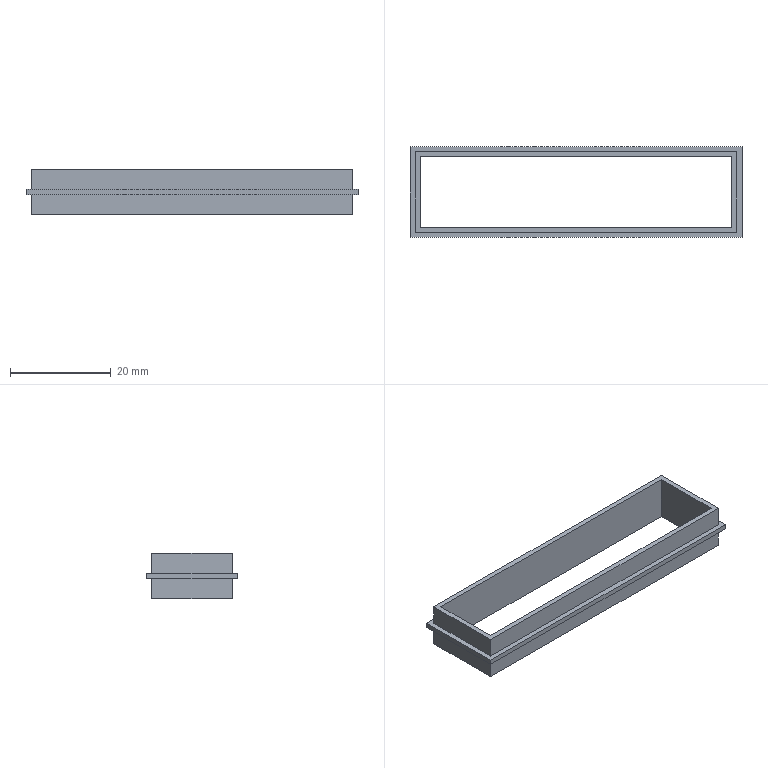Part | STEP file | 1-43.10 | 1 solid | 20 faces | box 66 x 18 x 9 mm | volume 1568 mm3 | plane 20
STEP:
#1=CARTESIAN_POINT('',(0.,0.,0.));
#2=DIRECTION('',(0.,0.,1.));
#3=DIRECTION('',(1.,0.,0.));
#4=AXIS2_PLACEMENT_3D('',#1,#2,#3);
#5=CARTESIAN_POINT('',(-32.,-8.,4.5));
#6=VERTEX_POINT('',#5);
#7=CARTESIAN_POINT('',(32.,-8.,4.5));
#8=VERTEX_POINT('',#7);
#9=CARTESIAN_POINT('',(-32.,-8.,4.5));
#10=DIRECTION('',(1.,0.,0.));
#11=VECTOR('',#10,1.);
#12=LINE('',#9,#11);
#13=CARTESIAN_POINT('',(0.,24.,4.5));
#14=DIRECTION('',(0.,0.,1.));
#15=DIRECTION('',(0.,1.,0.));
#16=AXIS2_PLACEMENT_3D('',#13,#14,#15);
#17=PLANE('',#16);
#18=CARTESIAN_POINT('',(-32.,32.));
#19=DIRECTION('',(0.,-1.));
#20=VECTOR('',#19,1.);
#21=LINE('',#18,#20);
#22=(GEOMETRIC_REPRESENTATION_CONTEXT(2)PARAMETRIC_REPRESENTATION_CONTEXT()REPRESENTATION_CONTEXT('',''));
#23=DEFINITIONAL_REPRESENTATION('',(#21),#22);
#24=PCURVE('',#17,#23);
#25=CARTESIAN_POINT('',(0.,-8.,0.));
#26=DIRECTION('',(0.,1.,0.));
#27=DIRECTION('',(1.,0.,0.));
#28=AXIS2_PLACEMENT_3D('',#25,#26,#27);
#29=PLANE('',#28);
#30=CARTESIAN_POINT('',(-32.,-4.5));
#31=DIRECTION('',(1.,0.));
#32=VECTOR('',#31,1.);
#33=LINE('',#30,#32);
#34=(GEOMETRIC_REPRESENTATION_CONTEXT(2)PARAMETRIC_REPRESENTATION_CONTEXT()REPRESENTATION_CONTEXT('',''));
#35=DEFINITIONAL_REPRESENTATION('',(#33),#34);
#36=PCURVE('',#29,#35);
#37=SURFACE_CURVE('',#12,(#24,#36),.PCURVE_S1.);
#38=EDGE_CURVE('',#6,#8,#37,.T.);
#39=ORIENTED_EDGE('',*,*,#38,.T.);
#40=CARTESIAN_POINT('',(32.,8.,4.5));
#41=VERTEX_POINT('',#40);
#42=CARTESIAN_POINT('',(32.,-8.,4.5));
#43=DIRECTION('',(0.,1.,0.));
#44=VECTOR('',#43,1.);
#45=LINE('',#42,#44);
#46=CARTESIAN_POINT('',(-32.,-32.));
#47=DIRECTION('',(1.,0.));
#48=VECTOR('',#47,1.);
#49=LINE('',#46,#48);
#50=(GEOMETRIC_REPRESENTATION_CONTEXT(2)PARAMETRIC_REPRESENTATION_CONTEXT()REPRESENTATION_CONTEXT('',''));
#51=DEFINITIONAL_REPRESENTATION('',(#49),#50);
#52=PCURVE('',#17,#51);
#53=CARTESIAN_POINT('',(32.,0.,0.));
#54=DIRECTION('',(-1.,0.,0.));
#55=DIRECTION('',(0.,1.,0.));
#56=AXIS2_PLACEMENT_3D('',#53,#54,#55);
#57=PLANE('',#56);
#58=CARTESIAN_POINT('',(-8.,-4.5));
#59=DIRECTION('',(1.,0.));
#60=VECTOR('',#59,1.);
#61=LINE('',#58,#60);
#62=(GEOMETRIC_REPRESENTATION_CONTEXT(2)PARAMETRIC_REPRESENTATION_CONTEXT()REPRESENTATION_CONTEXT('',''));
#63=DEFINITIONAL_REPRESENTATION('',(#61),#62);
#64=PCURVE('',#57,#63);
#65=SURFACE_CURVE('',#45,(#52,#64),.PCURVE_S1.);
#66=EDGE_CURVE('',#8,#41,#65,.T.);
#67=ORIENTED_EDGE('',*,*,#66,.T.);
#68=CARTESIAN_POINT('',(-32.,8.,4.5));
#69=VERTEX_POINT('',#68);
#70=CARTESIAN_POINT('',(32.,8.,4.5));
#71=DIRECTION('',(-1.,0.,0.));
#72=VECTOR('',#71,1.);
#73=LINE('',#70,#72);
#74=CARTESIAN_POINT('',(-16.,-32.));
#75=DIRECTION('',(0.,1.));
#76=VECTOR('',#75,1.);
#77=LINE('',#74,#76);
#78=(GEOMETRIC_REPRESENTATION_CONTEXT(2)PARAMETRIC_REPRESENTATION_CONTEXT()REPRESENTATION_CONTEXT('',''));
#79=DEFINITIONAL_REPRESENTATION('',(#77),#78);
#80=PCURVE('',#17,#79);
#81=CARTESIAN_POINT('',(0.,8.,0.));
#82=DIRECTION('',(0.,-1.,0.));
#83=DIRECTION('',(-1.,0.,0.));
#84=AXIS2_PLACEMENT_3D('',#81,#82,#83);
#85=PLANE('',#84);
#86=CARTESIAN_POINT('',(-32.,-4.5));
#87=DIRECTION('',(1.,0.));
#88=VECTOR('',#87,1.);
#89=LINE('',#86,#88);
#90=(GEOMETRIC_REPRESENTATION_CONTEXT(2)PARAMETRIC_REPRESENTATION_CONTEXT()REPRESENTATION_CONTEXT('',''));
#91=DEFINITIONAL_REPRESENTATION('',(#89),#90);
#92=PCURVE('',#85,#91);
#93=SURFACE_CURVE('',#73,(#80,#92),.PCURVE_S1.);
#94=EDGE_CURVE('',#41,#69,#93,.T.);
#95=ORIENTED_EDGE('',*,*,#94,.T.);
#96=CARTESIAN_POINT('',(-32.,8.,4.5));
#97=DIRECTION('',(0.,-1.,0.));
#98=VECTOR('',#97,1.);
#99=LINE('',#96,#98);
#100=CARTESIAN_POINT('',(-16.,32.));
#101=DIRECTION('',(-1.,0.));
#102=VECTOR('',#101,1.);
#103=LINE('',#100,#102);
#104=(GEOMETRIC_REPRESENTATION_CONTEXT(2)PARAMETRIC_REPRESENTATION_CONTEXT()REPRESENTATION_CONTEXT('',''));
#105=DEFINITIONAL_REPRESENTATION('',(#103),#104);
#106=PCURVE('',#17,#105);
#107=CARTESIAN_POINT('',(-32.,0.,0.));
#108=DIRECTION('',(1.,0.,0.));
#109=DIRECTION('',(0.,-1.,0.));
#110=AXIS2_PLACEMENT_3D('',#107,#108,#109);
#111=PLANE('',#110);
#112=CARTESIAN_POINT('',(-8.,-4.5));
#113=DIRECTION('',(1.,0.));
#114=VECTOR('',#113,1.);
#115=LINE('',#112,#114);
#116=(GEOMETRIC_REPRESENTATION_CONTEXT(2)PARAMETRIC_REPRESENTATION_CONTEXT()REPRESENTATION_CONTEXT('',''));
#117=DEFINITIONAL_REPRESENTATION('',(#115),#116);
#118=PCURVE('',#111,#117);
#119=SURFACE_CURVE('',#99,(#106,#118),.PCURVE_S1.);
#120=EDGE_CURVE('',#69,#6,#119,.T.);
#121=ORIENTED_EDGE('',*,*,#120,.T.);
#122=EDGE_LOOP('',(#39,#67,#95,#121));
#123=FACE_BOUND('',#122,.T.);
#124=CARTESIAN_POINT('',(31.,-7.,4.5));
#125=VERTEX_POINT('',#124);
#126=CARTESIAN_POINT('',(-31.,-7.,4.5));
#127=VERTEX_POINT('',#126);
#128=CARTESIAN_POINT('',(31.,-7.,4.5));
#129=DIRECTION('',(-1.,0.,0.));
#130=VECTOR('',#129,1.);
#131=LINE('',#128,#130);
#132=CARTESIAN_POINT('',(-31.,-31.));
#133=DIRECTION('',(0.,1.));
#134=VECTOR('',#133,1.);
#135=LINE('',#132,#134);
#136=(GEOMETRIC_REPRESENTATION_CONTEXT(2)PARAMETRIC_REPRESENTATION_CONTEXT()REPRESENTATION_CONTEXT('',''));
#137=DEFINITIONAL_REPRESENTATION('',(#135),#136);
#138=PCURVE('',#17,#137);
#139=CARTESIAN_POINT('',(0.,-7.,0.));
#140=DIRECTION('',(0.,-1.,0.));
#141=DIRECTION('',(-1.,0.,0.));
#142=AXIS2_PLACEMENT_3D('',#139,#140,#141);
#143=PLANE('',#142);
#144=CARTESIAN_POINT('',(-31.,-4.5));
#145=DIRECTION('',(1.,0.));
#146=VECTOR('',#145,1.);
#147=LINE('',#144,#146);
#148=(GEOMETRIC_REPRESENTATION_CONTEXT(2)PARAMETRIC_REPRESENTATION_CONTEXT()REPRESENTATION_CONTEXT('',''));
#149=DEFINITIONAL_REPRESENTATION('',(#147),#148);
#150=PCURVE('',#143,#149);
#151=SURFACE_CURVE('',#131,(#138,#150),.PCURVE_S1.);
#152=EDGE_CURVE('',#125,#127,#151,.T.);
#153=ORIENTED_EDGE('',*,*,#152,.T.);
#154=CARTESIAN_POINT('',(-31.,7.,4.5));
#155=VERTEX_POINT('',#154);
#156=CARTESIAN_POINT('',(-31.,-7.,4.5));
#157=DIRECTION('',(0.,1.,0.));
#158=VECTOR('',#157,1.);
#159=LINE('',#156,#158);
#160=CARTESIAN_POINT('',(-31.,31.));
#161=DIRECTION('',(1.,0.));
#162=VECTOR('',#161,1.);
#163=LINE('',#160,#162);
#164=(GEOMETRIC_REPRESENTATION_CONTEXT(2)PARAMETRIC_REPRESENTATION_CONTEXT()REPRESENTATION_CONTEXT('',''));
#165=DEFINITIONAL_REPRESENTATION('',(#163),#164);
#166=PCURVE('',#17,#165);
#167=CARTESIAN_POINT('',(-31.,0.,0.));
#168=DIRECTION('',(-1.,0.,0.));
#169=DIRECTION('',(0.,1.,0.));
#170=AXIS2_PLACEMENT_3D('',#167,#168,#169);
#171=PLANE('',#170);
#172=CARTESIAN_POINT('',(-7.,-4.5));
#173=DIRECTION('',(1.,0.));
#174=VECTOR('',#173,1.);
#175=LINE('',#172,#174);
#176=(GEOMETRIC_REPRESENTATION_CONTEXT(2)PARAMETRIC_REPRESENTATION_CONTEXT()REPRESENTATION_CONTEXT('',''));
#177=DEFINITIONAL_REPRESENTATION('',(#175),#176);
#178=PCURVE('',#171,#177);
#179=SURFACE_CURVE('',#159,(#166,#178),.PCURVE_S1.);
#180=EDGE_CURVE('',#127,#155,#179,.T.);
#181=ORIENTED_EDGE('',*,*,#180,.T.);
#182=CARTESIAN_POINT('',(31.,7.,4.5));
#183=VERTEX_POINT('',#182);
#184=CARTESIAN_POINT('',(-31.,7.,4.5));
#185=DIRECTION('',(1.,0.,0.));
#186=VECTOR('',#185,1.);
#187=LINE('',#184,#186);
#188=CARTESIAN_POINT('',(-17.,31.));
#189=DIRECTION('',(0.,-1.));
#190=VECTOR('',#189,1.);
#191=LINE('',#188,#190);
#192=(GEOMETRIC_REPRESENTATION_CONTEXT(2)PARAMETRIC_REPRESENTATION_CONTEXT()REPRESENTATION_CONTEXT('',''));
#193=DEFINITIONAL_REPRESENTATION('',(#191),#192);
#194=PCURVE('',#17,#193);
#195=CARTESIAN_POINT('',(0.,7.,0.));
#196=DIRECTION('',(0.,1.,0.));
#197=DIRECTION('',(1.,0.,0.));
#198=AXIS2_PLACEMENT_3D('',#195,#196,#197);
#199=PLANE('',#198);
#200=CARTESIAN_POINT('',(-31.,-4.5));
#201=DIRECTION('',(1.,0.));
#202=VECTOR('',#201,1.);
#203=LINE('',#200,#202);
#204=(GEOMETRIC_REPRESENTATION_CONTEXT(2)PARAMETRIC_REPRESENTATION_CONTEXT()REPRESENTATION_CONTEXT('',''));
#205=DEFINITIONAL_REPRESENTATION('',(#203),#204);
#206=PCURVE('',#199,#205);
#207=SURFACE_CURVE('',#187,(#194,#206),.PCURVE_S1.);
#208=EDGE_CURVE('',#155,#183,#207,.T.);
#209=ORIENTED_EDGE('',*,*,#208,.T.);
#210=CARTESIAN_POINT('',(31.,7.,4.5));
#211=DIRECTION('',(0.,-1.,0.));
#212=VECTOR('',#211,1.);
#213=LINE('',#210,#212);
#214=CARTESIAN_POINT('',(-17.,-31.));
#215=DIRECTION('',(-1.,0.));
#216=VECTOR('',#215,1.);
#217=LINE('',#214,#216);
#218=(GEOMETRIC_REPRESENTATION_CONTEXT(2)PARAMETRIC_REPRESENTATION_CONTEXT()REPRESENTATION_CONTEXT('',''));
#219=DEFINITIONAL_REPRESENTATION('',(#217),#218);
#220=PCURVE('',#17,#219);
#221=CARTESIAN_POINT('',(31.,0.,0.));
#222=DIRECTION('',(1.,0.,0.));
#223=DIRECTION('',(0.,-1.,0.));
#224=AXIS2_PLACEMENT_3D('',#221,#222,#223);
#225=PLANE('',#224);
#226=CARTESIAN_POINT('',(-7.,-4.5));
#227=DIRECTION('',(1.,0.));
#228=VECTOR('',#227,1.);
#229=LINE('',#226,#228);
#230=(GEOMETRIC_REPRESENTATION_CONTEXT(2)PARAMETRIC_REPRESENTATION_CONTEXT()REPRESENTATION_CONTEXT('',''));
#231=DEFINITIONAL_REPRESENTATION('',(#229),#230);
#232=PCURVE('',#225,#231);
#233=SURFACE_CURVE('',#213,(#220,#232),.PCURVE_S1.);
#234=EDGE_CURVE('',#183,#125,#233,.T.);
#235=ORIENTED_EDGE('',*,*,#234,.T.);
#236=EDGE_LOOP('',(#153,#181,#209,#235));
#237=FACE_BOUND('',#236,.T.);
#238=ADVANCED_FACE('',(#123,#237),#17,.T.);
#239=CARTESIAN_POINT('',(-32.,-8.,-4.5));
#240=VERTEX_POINT('',#239);
#241=CARTESIAN_POINT('',(32.,-8.,-4.5));
#242=VERTEX_POINT('',#241);
#243=CARTESIAN_POINT('',(-32.,-8.,-4.5));
#244=DIRECTION('',(1.,0.,0.));
#245=VECTOR('',#244,1.);
#246=LINE('',#243,#245);
#247=CARTESIAN_POINT('',(0.,24.,-4.5));
#248=DIRECTION('',(0.,0.,1.));
#249=DIRECTION('',(0.,1.,0.));
#250=AXIS2_PLACEMENT_3D('',#247,#248,#249);
#251=PLANE('',#250);
#252=CARTESIAN_POINT('',(-32.,32.));
#253=DIRECTION('',(0.,-1.));
#254=VECTOR('',#253,1.);
#255=LINE('',#252,#254);
#256=(GEOMETRIC_REPRESENTATION_CONTEXT(2)PARAMETRIC_REPRESENTATION_CONTEXT()REPRESENTATION_CONTEXT('',''));
#257=DEFINITIONAL_REPRESENTATION('',(#255),#256);
#258=PCURVE('',#251,#257);
#259=CARTESIAN_POINT('',(0.,-8.,0.));
#260=DIRECTION('',(0.,1.,0.));
#261=DIRECTION('',(1.,0.,0.));
#262=AXIS2_PLACEMENT_3D('',#259,#260,#261);
#263=PLANE('',#262);
#264=CARTESIAN_POINT('',(-32.,4.5));
#265=DIRECTION('',(1.,0.));
#266=VECTOR('',#265,1.);
#267=LINE('',#264,#266);
#268=(GEOMETRIC_REPRESENTATION_CONTEXT(2)PARAMETRIC_REPRESENTATION_CONTEXT()REPRESENTATION_CONTEXT('',''));
#269=DEFINITIONAL_REPRESENTATION('',(#267),#268);
#270=PCURVE('',#263,#269);
#271=SURFACE_CURVE('',#246,(#258,#270),.PCURVE_S1.);
#272=EDGE_CURVE('',#240,#242,#271,.T.);
#273=ORIENTED_EDGE('',*,*,#272,.T.);
#274=CARTESIAN_POINT('',(32.,8.,-4.5));
#275=VERTEX_POINT('',#274);
#276=CARTESIAN_POINT('',(32.,-8.,-4.5));
#277=DIRECTION('',(0.,1.,0.));
#278=VECTOR('',#277,1.);
#279=LINE('',#276,#278);
#280=CARTESIAN_POINT('',(-32.,-32.));
#281=DIRECTION('',(1.,0.));
#282=VECTOR('',#281,1.);
#283=LINE('',#280,#282);
#284=(GEOMETRIC_REPRESENTATION_CONTEXT(2)PARAMETRIC_REPRESENTATION_CONTEXT()REPRESENTATION_CONTEXT('',''));
#285=DEFINITIONAL_REPRESENTATION('',(#283),#284);
#286=PCURVE('',#251,#285);
#287=CARTESIAN_POINT('',(32.,0.,0.));
#288=DIRECTION('',(-1.,0.,0.));
#289=DIRECTION('',(0.,1.,0.));
#290=AXIS2_PLACEMENT_3D('',#287,#288,#289);
#291=PLANE('',#290);
#292=CARTESIAN_POINT('',(-8.,4.5));
#293=DIRECTION('',(1.,0.));
#294=VECTOR('',#293,1.);
#295=LINE('',#292,#294);
#296=(GEOMETRIC_REPRESENTATION_CONTEXT(2)PARAMETRIC_REPRESENTATION_CONTEXT()REPRESENTATION_CONTEXT('',''));
#297=DEFINITIONAL_REPRESENTATION('',(#295),#296);
#298=PCURVE('',#291,#297);
#299=SURFACE_CURVE('',#279,(#286,#298),.PCURVE_S1.);
#300=EDGE_CURVE('',#242,#275,#299,.T.);
#301=ORIENTED_EDGE('',*,*,#300,.T.);
#302=CARTESIAN_POINT('',(-32.,8.,-4.5));
#303=VERTEX_POINT('',#302);
#304=CARTESIAN_POINT('',(32.,8.,-4.5));
#305=DIRECTION('',(-1.,0.,0.));
#306=VECTOR('',#305,1.);
#307=LINE('',#304,#306);
#308=CARTESIAN_POINT('',(-16.,-32.));
#309=DIRECTION('',(0.,1.));
#310=VECTOR('',#309,1.);
#311=LINE('',#308,#310);
#312=(GEOMETRIC_REPRESENTATION_CONTEXT(2)PARAMETRIC_REPRESENTATION_CONTEXT()REPRESENTATION_CONTEXT('',''));
#313=DEFINITIONAL_REPRESENTATION('',(#311),#312);
#314=PCURVE('',#251,#313);
#315=CARTESIAN_POINT('',(0.,8.,0.));
#316=DIRECTION('',(0.,-1.,0.));
#317=DIRECTION('',(-1.,0.,0.));
#318=AXIS2_PLACEMENT_3D('',#315,#316,#317);
#319=PLANE('',#318);
#320=CARTESIAN_POINT('',(-32.,4.5));
#321=DIRECTION('',(1.,0.));
#322=VECTOR('',#321,1.);
#323=LINE('',#320,#322);
#324=(GEOMETRIC_REPRESENTATION_CONTEXT(2)PARAMETRIC_REPRESENTATION_CONTEXT()REPRESENTATION_CONTEXT('',''));
#325=DEFINITIONAL_REPRESENTATION('',(#323),#324);
#326=PCURVE('',#319,#325);
#327=SURFACE_CURVE('',#307,(#314,#326),.PCURVE_S1.);
#328=EDGE_CURVE('',#275,#303,#327,.T.);
#329=ORIENTED_EDGE('',*,*,#328,.T.);
#330=CARTESIAN_POINT('',(-32.,8.,-4.5));
#331=DIRECTION('',(0.,-1.,0.));
#332=VECTOR('',#331,1.);
#333=LINE('',#330,#332);
#334=CARTESIAN_POINT('',(-16.,32.));
#335=DIRECTION('',(-1.,0.));
#336=VECTOR('',#335,1.);
#337=LINE('',#334,#336);
#338=(GEOMETRIC_REPRESENTATION_CONTEXT(2)PARAMETRIC_REPRESENTATION_CONTEXT()REPRESENTATION_CONTEXT('',''));
#339=DEFINITIONAL_REPRESENTATION('',(#337),#338);
#340=PCURVE('',#251,#339);
#341=CARTESIAN_POINT('',(-32.,0.,0.));
#342=DIRECTION('',(1.,0.,0.));
#343=DIRECTION('',(0.,-1.,0.));
#344=AXIS2_PLACEMENT_3D('',#341,#342,#343);
#345=PLANE('',#344);
#346=CARTESIAN_POINT('',(-8.,4.5));
#347=DIRECTION('',(1.,0.));
#348=VECTOR('',#347,1.);
#349=LINE('',#346,#348);
#350=(GEOMETRIC_REPRESENTATION_CONTEXT(2)PARAMETRIC_REPRESENTATION_CONTEXT()REPRESENTATION_CONTEXT('',''));
#351=DEFINITIONAL_REPRESENTATION('',(#349),#350);
#352=PCURVE('',#345,#351);
#353=SURFACE_CURVE('',#333,(#340,#352),.PCURVE_S1.);
#354=EDGE_CURVE('',#303,#240,#353,.T.);
#355=ORIENTED_EDGE('',*,*,#354,.T.);
#356=EDGE_LOOP('',(#273,#301,#329,#355));
#357=FACE_BOUND('',#356,.F.);
#358=CARTESIAN_POINT('',(31.,-7.,-4.5));
#359=VERTEX_POINT('',#358);
#360=CARTESIAN_POINT('',(-31.,-7.,-4.5));
#361=VERTEX_POINT('',#360);
#362=CARTESIAN_POINT('',(31.,-7.,-4.5));
#363=DIRECTION('',(-1.,0.,0.));
#364=VECTOR('',#363,1.);
#365=LINE('',#362,#364);
#366=CARTESIAN_POINT('',(-31.,-31.));
#367=DIRECTION('',(0.,1.));
#368=VECTOR('',#367,1.);
#369=LINE('',#366,#368);
#370=(GEOMETRIC_REPRESENTATION_CONTEXT(2)PARAMETRIC_REPRESENTATION_CONTEXT()REPRESENTATION_CONTEXT('',''));
#371=DEFINITIONAL_REPRESENTATION('',(#369),#370);
#372=PCURVE('',#251,#371);
#373=CARTESIAN_POINT('',(-31.,4.5));
#374=DIRECTION('',(1.,0.));
#375=VECTOR('',#374,1.);
#376=LINE('',#373,#375);
#377=(GEOMETRIC_REPRESENTATION_CONTEXT(2)PARAMETRIC_REPRESENTATION_CONTEXT()REPRESENTATION_CONTEXT('',''));
#378=DEFINITIONAL_REPRESENTATION('',(#376),#377);
#379=PCURVE('',#143,#378);
#380=SURFACE_CURVE('',#365,(#372,#379),.PCURVE_S1.);
#381=EDGE_CURVE('',#359,#361,#380,.T.);
#382=ORIENTED_EDGE('',*,*,#381,.T.);
#383=CARTESIAN_POINT('',(-31.,7.,-4.5));
#384=VERTEX_POINT('',#383);
#385=CARTESIAN_POINT('',(-31.,-7.,-4.5));
#386=DIRECTION('',(0.,1.,0.));
#387=VECTOR('',#386,1.);
#388=LINE('',#385,#387);
#389=CARTESIAN_POINT('',(-31.,31.));
#390=DIRECTION('',(1.,0.));
#391=VECTOR('',#390,1.);
#392=LINE('',#389,#391);
#393=(GEOMETRIC_REPRESENTATION_CONTEXT(2)PARAMETRIC_REPRESENTATION_CONTEXT()REPRESENTATION_CONTEXT('',''));
#394=DEFINITIONAL_REPRESENTATION('',(#392),#393);
#395=PCURVE('',#251,#394);
#396=CARTESIAN_POINT('',(-7.,4.5));
#397=DIRECTION('',(1.,0.));
#398=VECTOR('',#397,1.);
#399=LINE('',#396,#398);
#400=(GEOMETRIC_REPRESENTATION_CONTEXT(2)PARAMETRIC_REPRESENTATION_CONTEXT()REPRESENTATION_CONTEXT('',''));
#401=DEFINITIONAL_REPRESENTATION('',(#399),#400);
#402=PCURVE('',#171,#401);
#403=SURFACE_CURVE('',#388,(#395,#402),.PCURVE_S1.);
#404=EDGE_CURVE('',#361,#384,#403,.T.);
#405=ORIENTED_EDGE('',*,*,#404,.T.);
#406=CARTESIAN_POINT('',(31.,7.,-4.5));
#407=VERTEX_POINT('',#406);
#408=CARTESIAN_POINT('',(-31.,7.,-4.5));
#409=DIRECTION('',(1.,0.,0.));
#410=VECTOR('',#409,1.);
#411=LINE('',#408,#410);
#412=CARTESIAN_POINT('',(-17.,31.));
#413=DIRECTION('',(0.,-1.));
#414=VECTOR('',#413,1.);
#415=LINE('',#412,#414);
#416=(GEOMETRIC_REPRESENTATION_CONTEXT(2)PARAMETRIC_REPRESENTATION_CONTEXT()REPRESENTATION_CONTEXT('',''));
#417=DEFINITIONAL_REPRESENTATION('',(#415),#416);
#418=PCURVE('',#251,#417);
#419=CARTESIAN_POINT('',(-31.,4.5));
#420=DIRECTION('',(1.,0.));
#421=VECTOR('',#420,1.);
#422=LINE('',#419,#421);
#423=(GEOMETRIC_REPRESENTATION_CONTEXT(2)PARAMETRIC_REPRESENTATION_CONTEXT()REPRESENTATION_CONTEXT('',''));
#424=DEFINITIONAL_REPRESENTATION('',(#422),#423);
#425=PCURVE('',#199,#424);
#426=SURFACE_CURVE('',#411,(#418,#425),.PCURVE_S1.);
#427=EDGE_CURVE('',#384,#407,#426,.T.);
#428=ORIENTED_EDGE('',*,*,#427,.T.);
#429=CARTESIAN_POINT('',(31.,7.,-4.5));
#430=DIRECTION('',(0.,-1.,0.));
#431=VECTOR('',#430,1.);
#432=LINE('',#429,#431);
#433=CARTESIAN_POINT('',(-17.,-31.));
#434=DIRECTION('',(-1.,0.));
#435=VECTOR('',#434,1.);
#436=LINE('',#433,#435);
#437=(GEOMETRIC_REPRESENTATION_CONTEXT(2)PARAMETRIC_REPRESENTATION_CONTEXT()REPRESENTATION_CONTEXT('',''));
#438=DEFINITIONAL_REPRESENTATION('',(#436),#437);
#439=PCURVE('',#251,#438);
#440=CARTESIAN_POINT('',(-7.,4.5));
#441=DIRECTION('',(1.,0.));
#442=VECTOR('',#441,1.);
#443=LINE('',#440,#442);
#444=(GEOMETRIC_REPRESENTATION_CONTEXT(2)PARAMETRIC_REPRESENTATION_CONTEXT()REPRESENTATION_CONTEXT('',''));
#445=DEFINITIONAL_REPRESENTATION('',(#443),#444);
#446=PCURVE('',#225,#445);
#447=SURFACE_CURVE('',#432,(#439,#446),.PCURVE_S1.);
#448=EDGE_CURVE('',#407,#359,#447,.T.);
#449=ORIENTED_EDGE('',*,*,#448,.T.);
#450=EDGE_LOOP('',(#382,#405,#428,#449));
#451=FACE_BOUND('',#450,.F.);
#452=ADVANCED_FACE('',(#357,#451),#251,.F.);
#453=ORIENTED_EDGE('',*,*,#152,.T.);
#454=CARTESIAN_POINT('',(-31.,-7.,4.5));
#455=DIRECTION('',(0.,0.,-1.));
#456=VECTOR('',#455,1.);
#457=LINE('',#454,#456);
#458=CARTESIAN_POINT('',(31.,-4.5));
#459=DIRECTION('',(0.,1.));
#460=VECTOR('',#459,1.);
#461=LINE('',#458,#460);
#462=(GEOMETRIC_REPRESENTATION_CONTEXT(2)PARAMETRIC_REPRESENTATION_CONTEXT()REPRESENTATION_CONTEXT('',''));
#463=DEFINITIONAL_REPRESENTATION('',(#461),#462);
#464=PCURVE('',#143,#463);
#465=CARTESIAN_POINT('',(-7.,-4.5));
#466=DIRECTION('',(0.,1.));
#467=VECTOR('',#466,1.);
#468=LINE('',#465,#467);
#469=(GEOMETRIC_REPRESENTATION_CONTEXT(2)PARAMETRIC_REPRESENTATION_CONTEXT()REPRESENTATION_CONTEXT('',''));
#470=DEFINITIONAL_REPRESENTATION('',(#468),#469);
#471=PCURVE('',#171,#470);
#472=SURFACE_CURVE('',#457,(#464,#471),.PCURVE_S1.);
#473=EDGE_CURVE('',#127,#361,#472,.T.);
#474=ORIENTED_EDGE('',*,*,#473,.T.);
#475=ORIENTED_EDGE('',*,*,#381,.F.);
#476=CARTESIAN_POINT('',(31.,-7.,4.5));
#477=DIRECTION('',(0.,0.,-1.));
#478=VECTOR('',#477,1.);
#479=LINE('',#476,#478);
#480=CARTESIAN_POINT('',(-31.,-4.5));
#481=DIRECTION('',(0.,1.));
#482=VECTOR('',#481,1.);
#483=LINE('',#480,#482);
#484=(GEOMETRIC_REPRESENTATION_CONTEXT(2)PARAMETRIC_REPRESENTATION_CONTEXT()REPRESENTATION_CONTEXT('',''));
#485=DEFINITIONAL_REPRESENTATION('',(#483),#484);
#486=PCURVE('',#143,#485);
#487=CARTESIAN_POINT('',(7.,-4.5));
#488=DIRECTION('',(0.,1.));
#489=VECTOR('',#488,1.);
#490=LINE('',#487,#489);
#491=(GEOMETRIC_REPRESENTATION_CONTEXT(2)PARAMETRIC_REPRESENTATION_CONTEXT()REPRESENTATION_CONTEXT('',''));
#492=DEFINITIONAL_REPRESENTATION('',(#490),#491);
#493=PCURVE('',#225,#492);
#494=SURFACE_CURVE('',#479,(#486,#493),.PCURVE_S1.);
#495=EDGE_CURVE('',#125,#359,#494,.T.);
#496=ORIENTED_EDGE('',*,*,#495,.F.);
#497=EDGE_LOOP('',(#453,#474,#475,#496));
#498=FACE_BOUND('',#497,.F.);
#499=ADVANCED_FACE('',(#498),#143,.F.);
#500=ORIENTED_EDGE('',*,*,#180,.T.);
#501=CARTESIAN_POINT('',(-31.,7.,4.5));
#502=DIRECTION('',(0.,0.,-1.));
#503=VECTOR('',#502,1.);
#504=LINE('',#501,#503);
#505=CARTESIAN_POINT('',(7.,-4.5));
#506=DIRECTION('',(0.,1.));
#507=VECTOR('',#506,1.);
#508=LINE('',#505,#507);
#509=(GEOMETRIC_REPRESENTATION_CONTEXT(2)PARAMETRIC_REPRESENTATION_CONTEXT()REPRESENTATION_CONTEXT('',''));
#510=DEFINITIONAL_REPRESENTATION('',(#508),#509);
#511=PCURVE('',#171,#510);
#512=CARTESIAN_POINT('',(-31.,-4.5));
#513=DIRECTION('',(0.,1.));
#514=VECTOR('',#513,1.);
#515=LINE('',#512,#514);
#516=(GEOMETRIC_REPRESENTATION_CONTEXT(2)PARAMETRIC_REPRESENTATION_CONTEXT()REPRESENTATION_CONTEXT('',''));
#517=DEFINITIONAL_REPRESENTATION('',(#515),#516);
#518=PCURVE('',#199,#517);
#519=SURFACE_CURVE('',#504,(#511,#518),.PCURVE_S1.);
#520=EDGE_CURVE('',#155,#384,#519,.T.);
#521=ORIENTED_EDGE('',*,*,#520,.T.);
#522=ORIENTED_EDGE('',*,*,#404,.F.);
#523=ORIENTED_EDGE('',*,*,#473,.F.);
#524=EDGE_LOOP('',(#500,#521,#522,#523));
#525=FACE_BOUND('',#524,.F.);
#526=ADVANCED_FACE('',(#525),#171,.F.);
#527=ORIENTED_EDGE('',*,*,#208,.T.);
#528=CARTESIAN_POINT('',(31.,7.,4.5));
#529=DIRECTION('',(0.,0.,-1.));
#530=VECTOR('',#529,1.);
#531=LINE('',#528,#530);
#532=CARTESIAN_POINT('',(31.,-4.5));
#533=DIRECTION('',(0.,1.));
#534=VECTOR('',#533,1.);
#535=LINE('',#532,#534);
#536=(GEOMETRIC_REPRESENTATION_CONTEXT(2)PARAMETRIC_REPRESENTATION_CONTEXT()REPRESENTATION_CONTEXT('',''));
#537=DEFINITIONAL_REPRESENTATION('',(#535),#536);
#538=PCURVE('',#199,#537);
#539=CARTESIAN_POINT('',(-7.,-4.5));
#540=DIRECTION('',(0.,1.));
#541=VECTOR('',#540,1.);
#542=LINE('',#539,#541);
#543=(GEOMETRIC_REPRESENTATION_CONTEXT(2)PARAMETRIC_REPRESENTATION_CONTEXT()REPRESENTATION_CONTEXT('',''));
#544=DEFINITIONAL_REPRESENTATION('',(#542),#543);
#545=PCURVE('',#225,#544);
#546=SURFACE_CURVE('',#531,(#538,#545),.PCURVE_S1.);
#547=EDGE_CURVE('',#183,#407,#546,.T.);
#548=ORIENTED_EDGE('',*,*,#547,.T.);
#549=ORIENTED_EDGE('',*,*,#427,.F.);
#550=ORIENTED_EDGE('',*,*,#520,.F.);
#551=EDGE_LOOP('',(#527,#548,#549,#550));
#552=FACE_BOUND('',#551,.F.);
#553=ADVANCED_FACE('',(#552),#199,.F.);
#554=ORIENTED_EDGE('',*,*,#234,.T.);
#555=ORIENTED_EDGE('',*,*,#495,.T.);
#556=ORIENTED_EDGE('',*,*,#448,.F.);
#557=ORIENTED_EDGE('',*,*,#547,.F.);
#558=EDGE_LOOP('',(#554,#555,#556,#557));
#559=FACE_BOUND('',#558,.F.);
#560=ADVANCED_FACE('',(#559),#225,.F.);
#561=ORIENTED_EDGE('',*,*,#38,.T.);
#562=CARTESIAN_POINT('',(32.,-8.,0.5));
#563=VERTEX_POINT('',#562);
#564=CARTESIAN_POINT('',(32.,-8.,4.5));
#565=DIRECTION('',(0.,0.,-1.));
#566=VECTOR('',#565,1.);
#567=LINE('',#564,#566);
#568=CARTESIAN_POINT('',(32.,-4.5));
#569=DIRECTION('',(0.,1.));
#570=VECTOR('',#569,1.);
#571=LINE('',#568,#570);
#572=(GEOMETRIC_REPRESENTATION_CONTEXT(2)PARAMETRIC_REPRESENTATION_CONTEXT()REPRESENTATION_CONTEXT('',''));
#573=DEFINITIONAL_REPRESENTATION('',(#571),#572);
#574=PCURVE('',#29,#573);
#575=CARTESIAN_POINT('',(-8.,-4.5));
#576=DIRECTION('',(0.,1.));
#577=VECTOR('',#576,1.);
#578=LINE('',#575,#577);
#579=(GEOMETRIC_REPRESENTATION_CONTEXT(2)PARAMETRIC_REPRESENTATION_CONTEXT()REPRESENTATION_CONTEXT('',''));
#580=DEFINITIONAL_REPRESENTATION('',(#578),#579);
#581=PCURVE('',#57,#580);
#582=SURFACE_CURVE('',#567,(#574,#581),.PCURVE_S1.);
#583=EDGE_CURVE('',#8,#563,#582,.T.);
#584=ORIENTED_EDGE('',*,*,#583,.T.);
#585=CARTESIAN_POINT('',(-32.,-8.,0.5));
#586=VERTEX_POINT('',#585);
#587=CARTESIAN_POINT('',(32.,-8.,0.5));
#588=DIRECTION('',(-1.,0.,0.));
#589=VECTOR('',#588,1.);
#590=LINE('',#587,#589);
#591=CARTESIAN_POINT('',(32.,-0.5));
#592=DIRECTION('',(-1.,0.));
#593=VECTOR('',#592,1.);
#594=LINE('',#591,#593);
#595=(GEOMETRIC_REPRESENTATION_CONTEXT(2)PARAMETRIC_REPRESENTATION_CONTEXT()REPRESENTATION_CONTEXT('',''));
#596=DEFINITIONAL_REPRESENTATION('',(#594),#595);
#597=PCURVE('',#29,#596);
#598=CARTESIAN_POINT('',(0.,24.,0.5));
#599=DIRECTION('',(0.,0.,1.));
#600=DIRECTION('',(0.,1.,0.));
#601=AXIS2_PLACEMENT_3D('',#598,#599,#600);
#602=PLANE('',#601);
#603=CARTESIAN_POINT('',(-32.,-32.));
#604=DIRECTION('',(0.,1.));
#605=VECTOR('',#604,1.);
#606=LINE('',#603,#605);
#607=(GEOMETRIC_REPRESENTATION_CONTEXT(2)PARAMETRIC_REPRESENTATION_CONTEXT()REPRESENTATION_CONTEXT('',''));
#608=DEFINITIONAL_REPRESENTATION('',(#606),#607);
#609=PCURVE('',#602,#608);
#610=SURFACE_CURVE('',#590,(#597,#609),.PCURVE_S1.);
#611=EDGE_CURVE('',#563,#586,#610,.T.);
#612=ORIENTED_EDGE('',*,*,#611,.T.);
#613=CARTESIAN_POINT('',(-32.,-8.,4.5));
#614=DIRECTION('',(0.,0.,-1.));
#615=VECTOR('',#614,1.);
#616=LINE('',#613,#615);
#617=CARTESIAN_POINT('',(-32.,-4.5));
#618=DIRECTION('',(0.,1.));
#619=VECTOR('',#618,1.);
#620=LINE('',#617,#619);
#621=(GEOMETRIC_REPRESENTATION_CONTEXT(2)PARAMETRIC_REPRESENTATION_CONTEXT()REPRESENTATION_CONTEXT('',''));
#622=DEFINITIONAL_REPRESENTATION('',(#620),#621);
#623=PCURVE('',#29,#622);
#624=CARTESIAN_POINT('',(8.,-4.5));
#625=DIRECTION('',(0.,1.));
#626=VECTOR('',#625,1.);
#627=LINE('',#624,#626);
#628=(GEOMETRIC_REPRESENTATION_CONTEXT(2)PARAMETRIC_REPRESENTATION_CONTEXT()REPRESENTATION_CONTEXT('',''));
#629=DEFINITIONAL_REPRESENTATION('',(#627),#628);
#630=PCURVE('',#111,#629);
#631=SURFACE_CURVE('',#616,(#623,#630),.PCURVE_S1.);
#632=EDGE_CURVE('',#6,#586,#631,.T.);
#633=ORIENTED_EDGE('',*,*,#632,.F.);
#634=EDGE_LOOP('',(#561,#584,#612,#633));
#635=FACE_BOUND('',#634,.F.);
#636=ADVANCED_FACE('',(#635),#29,.F.);
#637=ORIENTED_EDGE('',*,*,#272,.F.);
#638=CARTESIAN_POINT('',(-32.,-8.,-0.5));
#639=VERTEX_POINT('',#638);
#640=CARTESIAN_POINT('',(-32.,-8.,-0.5));
#641=DIRECTION('',(0.,0.,-1.));
#642=VECTOR('',#641,1.);
#643=LINE('',#640,#642);
#644=CARTESIAN_POINT('',(-32.,0.5));
#645=DIRECTION('',(0.,1.));
#646=VECTOR('',#645,1.);
#647=LINE('',#644,#646);
#648=(GEOMETRIC_REPRESENTATION_CONTEXT(2)PARAMETRIC_REPRESENTATION_CONTEXT()REPRESENTATION_CONTEXT('',''));
#649=DEFINITIONAL_REPRESENTATION('',(#647),#648);
#650=PCURVE('',#263,#649);
#651=CARTESIAN_POINT('',(8.,0.5));
#652=DIRECTION('',(0.,1.));
#653=VECTOR('',#652,1.);
#654=LINE('',#651,#653);
#655=(GEOMETRIC_REPRESENTATION_CONTEXT(2)PARAMETRIC_REPRESENTATION_CONTEXT()REPRESENTATION_CONTEXT('',''));
#656=DEFINITIONAL_REPRESENTATION('',(#654),#655);
#657=PCURVE('',#345,#656);
#658=SURFACE_CURVE('',#643,(#650,#657),.PCURVE_S1.);
#659=EDGE_CURVE('',#639,#240,#658,.T.);
#660=ORIENTED_EDGE('',*,*,#659,.F.);
#661=CARTESIAN_POINT('',(32.,-8.,-0.5));
#662=VERTEX_POINT('',#661);
#663=CARTESIAN_POINT('',(32.,-8.,-0.5));
#664=DIRECTION('',(-1.,0.,0.));
#665=VECTOR('',#664,1.);
#666=LINE('',#663,#665);
#667=CARTESIAN_POINT('',(32.,0.5));
#668=DIRECTION('',(-1.,0.));
#669=VECTOR('',#668,1.);
#670=LINE('',#667,#669);
#671=(GEOMETRIC_REPRESENTATION_CONTEXT(2)PARAMETRIC_REPRESENTATION_CONTEXT()REPRESENTATION_CONTEXT('',''));
#672=DEFINITIONAL_REPRESENTATION('',(#670),#671);
#673=PCURVE('',#263,#672);
#674=CARTESIAN_POINT('',(0.,24.,-0.5));
#675=DIRECTION('',(0.,0.,1.));
#676=DIRECTION('',(0.,1.,0.));
#677=AXIS2_PLACEMENT_3D('',#674,#675,#676);
#678=PLANE('',#677);
#679=CARTESIAN_POINT('',(-32.,-32.));
#680=DIRECTION('',(0.,1.));
#681=VECTOR('',#680,1.);
#682=LINE('',#679,#681);
#683=(GEOMETRIC_REPRESENTATION_CONTEXT(2)PARAMETRIC_REPRESENTATION_CONTEXT()REPRESENTATION_CONTEXT('',''));
#684=DEFINITIONAL_REPRESENTATION('',(#682),#683);
#685=PCURVE('',#678,#684);
#686=SURFACE_CURVE('',#666,(#673,#685),.PCURVE_S1.);
#687=EDGE_CURVE('',#662,#639,#686,.T.);
#688=ORIENTED_EDGE('',*,*,#687,.F.);
#689=CARTESIAN_POINT('',(32.,-8.,-0.5));
#690=DIRECTION('',(0.,0.,-1.));
#691=VECTOR('',#690,1.);
#692=LINE('',#689,#691);
#693=CARTESIAN_POINT('',(32.,0.5));
#694=DIRECTION('',(0.,1.));
#695=VECTOR('',#694,1.);
#696=LINE('',#693,#695);
#697=(GEOMETRIC_REPRESENTATION_CONTEXT(2)PARAMETRIC_REPRESENTATION_CONTEXT()REPRESENTATION_CONTEXT('',''));
#698=DEFINITIONAL_REPRESENTATION('',(#696),#697);
#699=PCURVE('',#263,#698);
#700=CARTESIAN_POINT('',(-8.,0.5));
#701=DIRECTION('',(0.,1.));
#702=VECTOR('',#701,1.);
#703=LINE('',#700,#702);
#704=(GEOMETRIC_REPRESENTATION_CONTEXT(2)PARAMETRIC_REPRESENTATION_CONTEXT()REPRESENTATION_CONTEXT('',''));
#705=DEFINITIONAL_REPRESENTATION('',(#703),#704);
#706=PCURVE('',#291,#705);
#707=SURFACE_CURVE('',#692,(#699,#706),.PCURVE_S1.);
#708=EDGE_CURVE('',#662,#242,#707,.T.);
#709=ORIENTED_EDGE('',*,*,#708,.T.);
#710=EDGE_LOOP('',(#637,#660,#688,#709));
#711=FACE_BOUND('',#710,.F.);
#712=ADVANCED_FACE('',(#711),#263,.F.);
#713=ORIENTED_EDGE('',*,*,#66,.T.);
#714=CARTESIAN_POINT('',(32.,8.,0.5));
#715=VERTEX_POINT('',#714);
#716=CARTESIAN_POINT('',(32.,8.,4.5));
#717=DIRECTION('',(0.,0.,-1.));
#718=VECTOR('',#717,1.);
#719=LINE('',#716,#718);
#720=CARTESIAN_POINT('',(8.,-4.5));
#721=DIRECTION('',(0.,1.));
#722=VECTOR('',#721,1.);
#723=LINE('',#720,#722);
#724=(GEOMETRIC_REPRESENTATION_CONTEXT(2)PARAMETRIC_REPRESENTATION_CONTEXT()REPRESENTATION_CONTEXT('',''));
#725=DEFINITIONAL_REPRESENTATION('',(#723),#724);
#726=PCURVE('',#57,#725);
#727=CARTESIAN_POINT('',(-32.,-4.5));
#728=DIRECTION('',(0.,1.));
#729=VECTOR('',#728,1.);
#730=LINE('',#727,#729);
#731=(GEOMETRIC_REPRESENTATION_CONTEXT(2)PARAMETRIC_REPRESENTATION_CONTEXT()REPRESENTATION_CONTEXT('',''));
#732=DEFINITIONAL_REPRESENTATION('',(#730),#731);
#733=PCURVE('',#85,#732);
#734=SURFACE_CURVE('',#719,(#726,#733),.PCURVE_S1.);
#735=EDGE_CURVE('',#41,#715,#734,.T.);
#736=ORIENTED_EDGE('',*,*,#735,.T.);
#737=CARTESIAN_POINT('',(32.,8.,0.5));
#738=DIRECTION('',(0.,-1.,0.));
#739=VECTOR('',#738,1.);
#740=LINE('',#737,#739);
#741=CARTESIAN_POINT('',(8.,-0.5));
#742=DIRECTION('',(-1.,0.));
#743=VECTOR('',#742,1.);
#744=LINE('',#741,#743);
#745=(GEOMETRIC_REPRESENTATION_CONTEXT(2)PARAMETRIC_REPRESENTATION_CONTEXT()REPRESENTATION_CONTEXT('',''));
#746=DEFINITIONAL_REPRESENTATION('',(#744),#745);
#747=PCURVE('',#57,#746);
#748=CARTESIAN_POINT('',(-16.,-32.));
#749=DIRECTION('',(-1.,0.));
#750=VECTOR('',#749,1.);
#751=LINE('',#748,#750);
#752=(GEOMETRIC_REPRESENTATION_CONTEXT(2)PARAMETRIC_REPRESENTATION_CONTEXT()REPRESENTATION_CONTEXT('',''));
#753=DEFINITIONAL_REPRESENTATION('',(#751),#752);
#754=PCURVE('',#602,#753);
#755=SURFACE_CURVE('',#740,(#747,#754),.PCURVE_S1.);
#756=EDGE_CURVE('',#715,#563,#755,.T.);
#757=ORIENTED_EDGE('',*,*,#756,.T.);
#758=ORIENTED_EDGE('',*,*,#583,.F.);
#759=EDGE_LOOP('',(#713,#736,#757,#758));
#760=FACE_BOUND('',#759,.F.);
#761=ADVANCED_FACE('',(#760),#57,.F.);
#762=ORIENTED_EDGE('',*,*,#300,.F.);
#763=ORIENTED_EDGE('',*,*,#708,.F.);
#764=CARTESIAN_POINT('',(32.,8.,-0.5));
#765=VERTEX_POINT('',#764);
#766=CARTESIAN_POINT('',(32.,8.,-0.5));
#767=DIRECTION('',(0.,-1.,0.));
#768=VECTOR('',#767,1.);
#769=LINE('',#766,#768);
#770=CARTESIAN_POINT('',(8.,0.5));
#771=DIRECTION('',(-1.,0.));
#772=VECTOR('',#771,1.);
#773=LINE('',#770,#772);
#774=(GEOMETRIC_REPRESENTATION_CONTEXT(2)PARAMETRIC_REPRESENTATION_CONTEXT()REPRESENTATION_CONTEXT('',''));
#775=DEFINITIONAL_REPRESENTATION('',(#773),#774);
#776=PCURVE('',#291,#775);
#777=CARTESIAN_POINT('',(-16.,-32.));
#778=DIRECTION('',(-1.,0.));
#779=VECTOR('',#778,1.);
#780=LINE('',#777,#779);
#781=(GEOMETRIC_REPRESENTATION_CONTEXT(2)PARAMETRIC_REPRESENTATION_CONTEXT()REPRESENTATION_CONTEXT('',''));
#782=DEFINITIONAL_REPRESENTATION('',(#780),#781);
#783=PCURVE('',#678,#782);
#784=SURFACE_CURVE('',#769,(#776,#783),.PCURVE_S1.);
#785=EDGE_CURVE('',#765,#662,#784,.T.);
#786=ORIENTED_EDGE('',*,*,#785,.F.);
#787=CARTESIAN_POINT('',(32.,8.,-0.5));
#788=DIRECTION('',(0.,0.,-1.));
#789=VECTOR('',#788,1.);
#790=LINE('',#787,#789);
#791=CARTESIAN_POINT('',(8.,0.5));
#792=DIRECTION('',(0.,1.));
#793=VECTOR('',#792,1.);
#794=LINE('',#791,#793);
#795=(GEOMETRIC_REPRESENTATION_CONTEXT(2)PARAMETRIC_REPRESENTATION_CONTEXT()REPRESENTATION_CONTEXT('',''));
#796=DEFINITIONAL_REPRESENTATION('',(#794),#795);
#797=PCURVE('',#291,#796);
#798=CARTESIAN_POINT('',(-32.,0.5));
#799=DIRECTION('',(0.,1.));
#800=VECTOR('',#799,1.);
#801=LINE('',#798,#800);
#802=(GEOMETRIC_REPRESENTATION_CONTEXT(2)PARAMETRIC_REPRESENTATION_CONTEXT()REPRESENTATION_CONTEXT('',''));
#803=DEFINITIONAL_REPRESENTATION('',(#801),#802);
#804=PCURVE('',#319,#803);
#805=SURFACE_CURVE('',#790,(#797,#804),.PCURVE_S1.);
#806=EDGE_CURVE('',#765,#275,#805,.T.);
#807=ORIENTED_EDGE('',*,*,#806,.T.);
#808=EDGE_LOOP('',(#762,#763,#786,#807));
#809=FACE_BOUND('',#808,.F.);
#810=ADVANCED_FACE('',(#809),#291,.F.);
#811=ORIENTED_EDGE('',*,*,#94,.T.);
#812=CARTESIAN_POINT('',(-32.,8.,0.5));
#813=VERTEX_POINT('',#812);
#814=CARTESIAN_POINT('',(-32.,8.,4.5));
#815=DIRECTION('',(0.,0.,-1.));
#816=VECTOR('',#815,1.);
#817=LINE('',#814,#816);
#818=CARTESIAN_POINT('',(32.,-4.5));
#819=DIRECTION('',(0.,1.));
#820=VECTOR('',#819,1.);
#821=LINE('',#818,#820);
#822=(GEOMETRIC_REPRESENTATION_CONTEXT(2)PARAMETRIC_REPRESENTATION_CONTEXT()REPRESENTATION_CONTEXT('',''));
#823=DEFINITIONAL_REPRESENTATION('',(#821),#822);
#824=PCURVE('',#85,#823);
#825=CARTESIAN_POINT('',(-8.,-4.5));
#826=DIRECTION('',(0.,1.));
#827=VECTOR('',#826,1.);
#828=LINE('',#825,#827);
#829=(GEOMETRIC_REPRESENTATION_CONTEXT(2)PARAMETRIC_REPRESENTATION_CONTEXT()REPRESENTATION_CONTEXT('',''));
#830=DEFINITIONAL_REPRESENTATION('',(#828),#829);
#831=PCURVE('',#111,#830);
#832=SURFACE_CURVE('',#817,(#824,#831),.PCURVE_S1.);
#833=EDGE_CURVE('',#69,#813,#832,.T.);
#834=ORIENTED_EDGE('',*,*,#833,.T.);
#835=CARTESIAN_POINT('',(-32.,8.,0.5));
#836=DIRECTION('',(1.,0.,0.));
#837=VECTOR('',#836,1.);
#838=LINE('',#835,#837);
#839=CARTESIAN_POINT('',(32.,-0.5));
#840=DIRECTION('',(-1.,0.));
#841=VECTOR('',#840,1.);
#842=LINE('',#839,#841);
#843=(GEOMETRIC_REPRESENTATION_CONTEXT(2)PARAMETRIC_REPRESENTATION_CONTEXT()REPRESENTATION_CONTEXT('',''));
#844=DEFINITIONAL_REPRESENTATION('',(#842),#843);
#845=PCURVE('',#85,#844);
#846=CARTESIAN_POINT('',(-16.,32.));
#847=DIRECTION('',(0.,-1.));
#848=VECTOR('',#847,1.);
#849=LINE('',#846,#848);
#850=(GEOMETRIC_REPRESENTATION_CONTEXT(2)PARAMETRIC_REPRESENTATION_CONTEXT()REPRESENTATION_CONTEXT('',''));
#851=DEFINITIONAL_REPRESENTATION('',(#849),#850);
#852=PCURVE('',#602,#851);
#853=SURFACE_CURVE('',#838,(#845,#852),.PCURVE_S1.);
#854=EDGE_CURVE('',#813,#715,#853,.T.);
#855=ORIENTED_EDGE('',*,*,#854,.T.);
#856=ORIENTED_EDGE('',*,*,#735,.F.);
#857=EDGE_LOOP('',(#811,#834,#855,#856));
#858=FACE_BOUND('',#857,.F.);
#859=ADVANCED_FACE('',(#858),#85,.F.);
#860=ORIENTED_EDGE('',*,*,#328,.F.);
#861=ORIENTED_EDGE('',*,*,#806,.F.);
#862=CARTESIAN_POINT('',(-32.,8.,-0.5));
#863=VERTEX_POINT('',#862);
#864=CARTESIAN_POINT('',(-32.,8.,-0.5));
#865=DIRECTION('',(1.,0.,0.));
#866=VECTOR('',#865,1.);
#867=LINE('',#864,#866);
#868=CARTESIAN_POINT('',(32.,0.5));
#869=DIRECTION('',(-1.,0.));
#870=VECTOR('',#869,1.);
#871=LINE('',#868,#870);
#872=(GEOMETRIC_REPRESENTATION_CONTEXT(2)PARAMETRIC_REPRESENTATION_CONTEXT()REPRESENTATION_CONTEXT('',''));
#873=DEFINITIONAL_REPRESENTATION('',(#871),#872);
#874=PCURVE('',#319,#873);
#875=CARTESIAN_POINT('',(-16.,32.));
#876=DIRECTION('',(0.,-1.));
#877=VECTOR('',#876,1.);
#878=LINE('',#875,#877);
#879=(GEOMETRIC_REPRESENTATION_CONTEXT(2)PARAMETRIC_REPRESENTATION_CONTEXT()REPRESENTATION_CONTEXT('',''));
#880=DEFINITIONAL_REPRESENTATION('',(#878),#879);
#881=PCURVE('',#678,#880);
#882=SURFACE_CURVE('',#867,(#874,#881),.PCURVE_S1.);
#883=EDGE_CURVE('',#863,#765,#882,.T.);
#884=ORIENTED_EDGE('',*,*,#883,.F.);
#885=CARTESIAN_POINT('',(-32.,8.,-0.5));
#886=DIRECTION('',(0.,0.,-1.));
#887=VECTOR('',#886,1.);
#888=LINE('',#885,#887);
#889=CARTESIAN_POINT('',(32.,0.5));
#890=DIRECTION('',(0.,1.));
#891=VECTOR('',#890,1.);
#892=LINE('',#889,#891);
#893=(GEOMETRIC_REPRESENTATION_CONTEXT(2)PARAMETRIC_REPRESENTATION_CONTEXT()REPRESENTATION_CONTEXT('',''));
#894=DEFINITIONAL_REPRESENTATION('',(#892),#893);
#895=PCURVE('',#319,#894);
#896=CARTESIAN_POINT('',(-8.,0.5));
#897=DIRECTION('',(0.,1.));
#898=VECTOR('',#897,1.);
#899=LINE('',#896,#898);
#900=(GEOMETRIC_REPRESENTATION_CONTEXT(2)PARAMETRIC_REPRESENTATION_CONTEXT()REPRESENTATION_CONTEXT('',''));
#901=DEFINITIONAL_REPRESENTATION('',(#899),#900);
#902=PCURVE('',#345,#901);
#903=SURFACE_CURVE('',#888,(#895,#902),.PCURVE_S1.);
#904=EDGE_CURVE('',#863,#303,#903,.T.);
#905=ORIENTED_EDGE('',*,*,#904,.T.);
#906=EDGE_LOOP('',(#860,#861,#884,#905));
#907=FACE_BOUND('',#906,.F.);
#908=ADVANCED_FACE('',(#907),#319,.F.);
#909=ORIENTED_EDGE('',*,*,#120,.T.);
#910=ORIENTED_EDGE('',*,*,#632,.T.);
#911=CARTESIAN_POINT('',(-32.,-8.,0.5));
#912=DIRECTION('',(0.,1.,0.));
#913=VECTOR('',#912,1.);
#914=LINE('',#911,#913);
#915=CARTESIAN_POINT('',(8.,-0.5));
#916=DIRECTION('',(-1.,0.));
#917=VECTOR('',#916,1.);
#918=LINE('',#915,#917);
#919=(GEOMETRIC_REPRESENTATION_CONTEXT(2)PARAMETRIC_REPRESENTATION_CONTEXT()REPRESENTATION_CONTEXT('',''));
#920=DEFINITIONAL_REPRESENTATION('',(#918),#919);
#921=PCURVE('',#111,#920);
#922=CARTESIAN_POINT('',(-32.,32.));
#923=DIRECTION('',(1.,0.));
#924=VECTOR('',#923,1.);
#925=LINE('',#922,#924);
#926=(GEOMETRIC_REPRESENTATION_CONTEXT(2)PARAMETRIC_REPRESENTATION_CONTEXT()REPRESENTATION_CONTEXT('',''));
#927=DEFINITIONAL_REPRESENTATION('',(#925),#926);
#928=PCURVE('',#602,#927);
#929=SURFACE_CURVE('',#914,(#921,#928),.PCURVE_S1.);
#930=EDGE_CURVE('',#586,#813,#929,.T.);
#931=ORIENTED_EDGE('',*,*,#930,.T.);
#932=ORIENTED_EDGE('',*,*,#833,.F.);
#933=EDGE_LOOP('',(#909,#910,#931,#932));
#934=FACE_BOUND('',#933,.F.);
#935=ADVANCED_FACE('',(#934),#111,.F.);
#936=ORIENTED_EDGE('',*,*,#354,.F.);
#937=ORIENTED_EDGE('',*,*,#904,.F.);
#938=CARTESIAN_POINT('',(-32.,-8.,-0.5));
#939=DIRECTION('',(0.,1.,0.));
#940=VECTOR('',#939,1.);
#941=LINE('',#938,#940);
#942=CARTESIAN_POINT('',(8.,0.5));
#943=DIRECTION('',(-1.,0.));
#944=VECTOR('',#943,1.);
#945=LINE('',#942,#944);
#946=(GEOMETRIC_REPRESENTATION_CONTEXT(2)PARAMETRIC_REPRESENTATION_CONTEXT()REPRESENTATION_CONTEXT('',''));
#947=DEFINITIONAL_REPRESENTATION('',(#945),#946);
#948=PCURVE('',#345,#947);
#949=CARTESIAN_POINT('',(-32.,32.));
#950=DIRECTION('',(1.,0.));
#951=VECTOR('',#950,1.);
#952=LINE('',#949,#951);
#953=(GEOMETRIC_REPRESENTATION_CONTEXT(2)PARAMETRIC_REPRESENTATION_CONTEXT()REPRESENTATION_CONTEXT('',''));
#954=DEFINITIONAL_REPRESENTATION('',(#952),#953);
#955=PCURVE('',#678,#954);
#956=SURFACE_CURVE('',#941,(#948,#955),.PCURVE_S1.);
#957=EDGE_CURVE('',#639,#863,#956,.T.);
#958=ORIENTED_EDGE('',*,*,#957,.F.);
#959=ORIENTED_EDGE('',*,*,#659,.T.);
#960=EDGE_LOOP('',(#936,#937,#958,#959));
#961=FACE_BOUND('',#960,.F.);
#962=ADVANCED_FACE('',(#961),#345,.F.);
#963=CARTESIAN_POINT('',(33.,-9.,0.5));
#964=VERTEX_POINT('',#963);
#965=CARTESIAN_POINT('',(33.,9.,0.5));
#966=VERTEX_POINT('',#965);
#967=CARTESIAN_POINT('',(33.,-9.,0.5));
#968=DIRECTION('',(0.,1.,0.));
#969=VECTOR('',#968,1.);
#970=LINE('',#967,#969);
#971=CARTESIAN_POINT('',(-33.,-33.));
#972=DIRECTION('',(1.,0.));
#973=VECTOR('',#972,1.);
#974=LINE('',#971,#973);
#975=(GEOMETRIC_REPRESENTATION_CONTEXT(2)PARAMETRIC_REPRESENTATION_CONTEXT()REPRESENTATION_CONTEXT('',''));
#976=DEFINITIONAL_REPRESENTATION('',(#974),#975);
#977=PCURVE('',#602,#976);
#978=CARTESIAN_POINT('',(33.,0.,0.));
#979=DIRECTION('',(-1.,0.,0.));
#980=DIRECTION('',(0.,1.,0.));
#981=AXIS2_PLACEMENT_3D('',#978,#979,#980);
#982=PLANE('',#981);
#983=CARTESIAN_POINT('',(-9.,-0.5));
#984=DIRECTION('',(1.,0.));
#985=VECTOR('',#984,1.);
#986=LINE('',#983,#985);
#987=(GEOMETRIC_REPRESENTATION_CONTEXT(2)PARAMETRIC_REPRESENTATION_CONTEXT()REPRESENTATION_CONTEXT('',''));
#988=DEFINITIONAL_REPRESENTATION('',(#986),#987);
#989=PCURVE('',#982,#988);
#990=SURFACE_CURVE('',#970,(#977,#989),.PCURVE_S1.);
#991=EDGE_CURVE('',#964,#966,#990,.T.);
#992=ORIENTED_EDGE('',*,*,#991,.T.);
#993=CARTESIAN_POINT('',(-33.,9.,0.5));
#994=VERTEX_POINT('',#993);
#995=CARTESIAN_POINT('',(33.,9.,0.5));
#996=DIRECTION('',(-1.,0.,0.));
#997=VECTOR('',#996,1.);
#998=LINE('',#995,#997);
#999=CARTESIAN_POINT('',(-15.,-33.));
#1000=DIRECTION('',(0.,1.));
#1001=VECTOR('',#1000,1.);
#1002=LINE('',#999,#1001);
#1003=(GEOMETRIC_REPRESENTATION_CONTEXT(2)PARAMETRIC_REPRESENTATION_CONTEXT()REPRESENTATION_CONTEXT('',''));
#1004=DEFINITIONAL_REPRESENTATION('',(#1002),#1003);
#1005=PCURVE('',#602,#1004);
#1006=CARTESIAN_POINT('',(0.,9.,0.));
#1007=DIRECTION('',(0.,-1.,0.));
#1008=DIRECTION('',(-1.,0.,0.));
#1009=AXIS2_PLACEMENT_3D('',#1006,#1007,#1008);
#1010=PLANE('',#1009);
#1011=CARTESIAN_POINT('',(-33.,-0.5));
#1012=DIRECTION('',(1.,0.));
#1013=VECTOR('',#1012,1.);
#1014=LINE('',#1011,#1013);
#1015=(GEOMETRIC_REPRESENTATION_CONTEXT(2)PARAMETRIC_REPRESENTATION_CONTEXT()REPRESENTATION_CONTEXT('',''));
#1016=DEFINITIONAL_REPRESENTATION('',(#1014),#1015);
#1017=PCURVE('',#1010,#1016);
#1018=SURFACE_CURVE('',#998,(#1005,#1017),.PCURVE_S1.);
#1019=EDGE_CURVE('',#966,#994,#1018,.T.);
#1020=ORIENTED_EDGE('',*,*,#1019,.T.);
#1021=CARTESIAN_POINT('',(-33.,-9.,0.5));
#1022=VERTEX_POINT('',#1021);
#1023=CARTESIAN_POINT('',(-33.,9.,0.5));
#1024=DIRECTION('',(0.,-1.,0.));
#1025=VECTOR('',#1024,1.);
#1026=LINE('',#1023,#1025);
#1027=CARTESIAN_POINT('',(-15.,33.));
#1028=DIRECTION('',(-1.,0.));
#1029=VECTOR('',#1028,1.);
#1030=LINE('',#1027,#1029);
#1031=(GEOMETRIC_REPRESENTATION_CONTEXT(2)PARAMETRIC_REPRESENTATION_CONTEXT()REPRESENTATION_CONTEXT('',''));
#1032=DEFINITIONAL_REPRESENTATION('',(#1030),#1031);
#1033=PCURVE('',#602,#1032);
#1034=CARTESIAN_POINT('',(-33.,0.,0.));
#1035=DIRECTION('',(1.,0.,0.));
#1036=DIRECTION('',(0.,-1.,0.));
#1037=AXIS2_PLACEMENT_3D('',#1034,#1035,#1036);
#1038=PLANE('',#1037);
#1039=CARTESIAN_POINT('',(-9.,-0.5));
#1040=DIRECTION('',(1.,0.));
#1041=VECTOR('',#1040,1.);
#1042=LINE('',#1039,#1041);
#1043=(GEOMETRIC_REPRESENTATION_CONTEXT(2)PARAMETRIC_REPRESENTATION_CONTEXT()REPRESENTATION_CONTEXT('',''));
#1044=DEFINITIONAL_REPRESENTATION('',(#1042),#1043);
#1045=PCURVE('',#1038,#1044);
#1046=SURFACE_CURVE('',#1026,(#1033,#1045),.PCURVE_S1.);
#1047=EDGE_CURVE('',#994,#1022,#1046,.T.);
#1048=ORIENTED_EDGE('',*,*,#1047,.T.);
#1049=CARTESIAN_POINT('',(-33.,-9.,0.5));
#1050=DIRECTION('',(1.,0.,0.));
#1051=VECTOR('',#1050,1.);
#1052=LINE('',#1049,#1051);
#1053=CARTESIAN_POINT('',(-33.,33.));
#1054=DIRECTION('',(0.,-1.));
#1055=VECTOR('',#1054,1.);
#1056=LINE('',#1053,#1055);
#1057=(GEOMETRIC_REPRESENTATION_CONTEXT(2)PARAMETRIC_REPRESENTATION_CONTEXT()REPRESENTATION_CONTEXT('',''));
#1058=DEFINITIONAL_REPRESENTATION('',(#1056),#1057);
#1059=PCURVE('',#602,#1058);
#1060=CARTESIAN_POINT('',(0.,-9.,0.));
#1061=DIRECTION('',(0.,1.,0.));
#1062=DIRECTION('',(1.,0.,0.));
#1063=AXIS2_PLACEMENT_3D('',#1060,#1061,#1062);
#1064=PLANE('',#1063);
#1065=CARTESIAN_POINT('',(-33.,-0.5));
#1066=DIRECTION('',(1.,0.));
#1067=VECTOR('',#1066,1.);
#1068=LINE('',#1065,#1067);
#1069=(GEOMETRIC_REPRESENTATION_CONTEXT(2)PARAMETRIC_REPRESENTATION_CONTEXT()REPRESENTATION_CONTEXT('',''));
#1070=DEFINITIONAL_REPRESENTATION('',(#1068),#1069);
#1071=PCURVE('',#1064,#1070);
#1072=SURFACE_CURVE('',#1052,(#1059,#1071),.PCURVE_S1.);
#1073=EDGE_CURVE('',#1022,#964,#1072,.T.);
#1074=ORIENTED_EDGE('',*,*,#1073,.T.);
#1075=EDGE_LOOP('',(#992,#1020,#1048,#1074));
#1076=FACE_BOUND('',#1075,.T.);
#1077=ORIENTED_EDGE('',*,*,#611,.T.);
#1078=ORIENTED_EDGE('',*,*,#930,.T.);
#1079=ORIENTED_EDGE('',*,*,#854,.T.);
#1080=ORIENTED_EDGE('',*,*,#756,.T.);
#1081=EDGE_LOOP('',(#1077,#1078,#1079,#1080));
#1082=FACE_BOUND('',#1081,.T.);
#1083=ADVANCED_FACE('',(#1076,#1082),#602,.T.);
#1084=ORIENTED_EDGE('',*,*,#991,.T.);
#1085=CARTESIAN_POINT('',(33.,9.,-0.5));
#1086=VERTEX_POINT('',#1085);
#1087=CARTESIAN_POINT('',(33.,9.,0.5));
#1088=DIRECTION('',(0.,0.,-1.));
#1089=VECTOR('',#1088,1.);
#1090=LINE('',#1087,#1089);
#1091=CARTESIAN_POINT('',(9.,-0.5));
#1092=DIRECTION('',(0.,1.));
#1093=VECTOR('',#1092,1.);
#1094=LINE('',#1091,#1093);
#1095=(GEOMETRIC_REPRESENTATION_CONTEXT(2)PARAMETRIC_REPRESENTATION_CONTEXT()REPRESENTATION_CONTEXT('',''));
#1096=DEFINITIONAL_REPRESENTATION('',(#1094),#1095);
#1097=PCURVE('',#982,#1096);
#1098=CARTESIAN_POINT('',(-33.,-0.5));
#1099=DIRECTION('',(0.,1.));
#1100=VECTOR('',#1099,1.);
#1101=LINE('',#1098,#1100);
#1102=(GEOMETRIC_REPRESENTATION_CONTEXT(2)PARAMETRIC_REPRESENTATION_CONTEXT()REPRESENTATION_CONTEXT('',''));
#1103=DEFINITIONAL_REPRESENTATION('',(#1101),#1102);
#1104=PCURVE('',#1010,#1103);
#1105=SURFACE_CURVE('',#1090,(#1097,#1104),.PCURVE_S1.);
#1106=EDGE_CURVE('',#966,#1086,#1105,.T.);
#1107=ORIENTED_EDGE('',*,*,#1106,.T.);
#1108=CARTESIAN_POINT('',(33.,-9.,-0.5));
#1109=VERTEX_POINT('',#1108);
#1110=CARTESIAN_POINT('',(33.,-9.,-0.5));
#1111=DIRECTION('',(0.,1.,0.));
#1112=VECTOR('',#1111,1.);
#1113=LINE('',#1110,#1112);
#1114=CARTESIAN_POINT('',(-9.,0.5));
#1115=DIRECTION('',(1.,0.));
#1116=VECTOR('',#1115,1.);
#1117=LINE('',#1114,#1116);
#1118=(GEOMETRIC_REPRESENTATION_CONTEXT(2)PARAMETRIC_REPRESENTATION_CONTEXT()REPRESENTATION_CONTEXT('',''));
#1119=DEFINITIONAL_REPRESENTATION('',(#1117),#1118);
#1120=PCURVE('',#982,#1119);
#1121=CARTESIAN_POINT('',(-33.,-33.));
#1122=DIRECTION('',(1.,0.));
#1123=VECTOR('',#1122,1.);
#1124=LINE('',#1121,#1123);
#1125=(GEOMETRIC_REPRESENTATION_CONTEXT(2)PARAMETRIC_REPRESENTATION_CONTEXT()REPRESENTATION_CONTEXT('',''));
#1126=DEFINITIONAL_REPRESENTATION('',(#1124),#1125);
#1127=PCURVE('',#678,#1126);
#1128=SURFACE_CURVE('',#1113,(#1120,#1127),.PCURVE_S1.);
#1129=EDGE_CURVE('',#1109,#1086,#1128,.T.);
#1130=ORIENTED_EDGE('',*,*,#1129,.F.);
#1131=CARTESIAN_POINT('',(33.,-9.,0.5));
#1132=DIRECTION('',(0.,0.,-1.));
#1133=VECTOR('',#1132,1.);
#1134=LINE('',#1131,#1133);
#1135=CARTESIAN_POINT('',(-9.,-0.5));
#1136=DIRECTION('',(0.,1.));
#1137=VECTOR('',#1136,1.);
#1138=LINE('',#1135,#1137);
#1139=(GEOMETRIC_REPRESENTATION_CONTEXT(2)PARAMETRIC_REPRESENTATION_CONTEXT()REPRESENTATION_CONTEXT('',''));
#1140=DEFINITIONAL_REPRESENTATION('',(#1138),#1139);
#1141=PCURVE('',#982,#1140);
#1142=CARTESIAN_POINT('',(33.,-0.5));
#1143=DIRECTION('',(0.,1.));
#1144=VECTOR('',#1143,1.);
#1145=LINE('',#1142,#1144);
#1146=(GEOMETRIC_REPRESENTATION_CONTEXT(2)PARAMETRIC_REPRESENTATION_CONTEXT()REPRESENTATION_CONTEXT('',''));
#1147=DEFINITIONAL_REPRESENTATION('',(#1145),#1146);
#1148=PCURVE('',#1064,#1147);
#1149=SURFACE_CURVE('',#1134,(#1141,#1148),.PCURVE_S1.);
#1150=EDGE_CURVE('',#964,#1109,#1149,.T.);
#1151=ORIENTED_EDGE('',*,*,#1150,.F.);
#1152=EDGE_LOOP('',(#1084,#1107,#1130,#1151));
#1153=FACE_BOUND('',#1152,.F.);
#1154=ADVANCED_FACE('',(#1153),#982,.F.);
#1155=ORIENTED_EDGE('',*,*,#1019,.T.);
#1156=CARTESIAN_POINT('',(-33.,9.,-0.5));
#1157=VERTEX_POINT('',#1156);
#1158=CARTESIAN_POINT('',(-33.,9.,0.5));
#1159=DIRECTION('',(0.,0.,-1.));
#1160=VECTOR('',#1159,1.);
#1161=LINE('',#1158,#1160);
#1162=CARTESIAN_POINT('',(33.,-0.5));
#1163=DIRECTION('',(0.,1.));
#1164=VECTOR('',#1163,1.);
#1165=LINE('',#1162,#1164);
#1166=(GEOMETRIC_REPRESENTATION_CONTEXT(2)PARAMETRIC_REPRESENTATION_CONTEXT()REPRESENTATION_CONTEXT('',''));
#1167=DEFINITIONAL_REPRESENTATION('',(#1165),#1166);
#1168=PCURVE('',#1010,#1167);
#1169=CARTESIAN_POINT('',(-9.,-0.5));
#1170=DIRECTION('',(0.,1.));
#1171=VECTOR('',#1170,1.);
#1172=LINE('',#1169,#1171);
#1173=(GEOMETRIC_REPRESENTATION_CONTEXT(2)PARAMETRIC_REPRESENTATION_CONTEXT()REPRESENTATION_CONTEXT('',''));
#1174=DEFINITIONAL_REPRESENTATION('',(#1172),#1173);
#1175=PCURVE('',#1038,#1174);
#1176=SURFACE_CURVE('',#1161,(#1168,#1175),.PCURVE_S1.);
#1177=EDGE_CURVE('',#994,#1157,#1176,.T.);
#1178=ORIENTED_EDGE('',*,*,#1177,.T.);
#1179=CARTESIAN_POINT('',(33.,9.,-0.5));
#1180=DIRECTION('',(-1.,0.,0.));
#1181=VECTOR('',#1180,1.);
#1182=LINE('',#1179,#1181);
#1183=CARTESIAN_POINT('',(-33.,0.5));
#1184=DIRECTION('',(1.,0.));
#1185=VECTOR('',#1184,1.);
#1186=LINE('',#1183,#1185);
#1187=(GEOMETRIC_REPRESENTATION_CONTEXT(2)PARAMETRIC_REPRESENTATION_CONTEXT()REPRESENTATION_CONTEXT('',''));
#1188=DEFINITIONAL_REPRESENTATION('',(#1186),#1187);
#1189=PCURVE('',#1010,#1188);
#1190=CARTESIAN_POINT('',(-15.,-33.));
#1191=DIRECTION('',(0.,1.));
#1192=VECTOR('',#1191,1.);
#1193=LINE('',#1190,#1192);
#1194=(GEOMETRIC_REPRESENTATION_CONTEXT(2)PARAMETRIC_REPRESENTATION_CONTEXT()REPRESENTATION_CONTEXT('',''));
#1195=DEFINITIONAL_REPRESENTATION('',(#1193),#1194);
#1196=PCURVE('',#678,#1195);
#1197=SURFACE_CURVE('',#1182,(#1189,#1196),.PCURVE_S1.);
#1198=EDGE_CURVE('',#1086,#1157,#1197,.T.);
#1199=ORIENTED_EDGE('',*,*,#1198,.F.);
#1200=ORIENTED_EDGE('',*,*,#1106,.F.);
#1201=EDGE_LOOP('',(#1155,#1178,#1199,#1200));
#1202=FACE_BOUND('',#1201,.F.);
#1203=ADVANCED_FACE('',(#1202),#1010,.F.);
#1204=ORIENTED_EDGE('',*,*,#1047,.T.);
#1205=CARTESIAN_POINT('',(-33.,-9.,-0.5));
#1206=VERTEX_POINT('',#1205);
#1207=CARTESIAN_POINT('',(-33.,-9.,0.5));
#1208=DIRECTION('',(0.,0.,-1.));
#1209=VECTOR('',#1208,1.);
#1210=LINE('',#1207,#1209);
#1211=CARTESIAN_POINT('',(9.,-0.5));
#1212=DIRECTION('',(0.,1.));
#1213=VECTOR('',#1212,1.);
#1214=LINE('',#1211,#1213);
#1215=(GEOMETRIC_REPRESENTATION_CONTEXT(2)PARAMETRIC_REPRESENTATION_CONTEXT()REPRESENTATION_CONTEXT('',''));
#1216=DEFINITIONAL_REPRESENTATION('',(#1214),#1215);
#1217=PCURVE('',#1038,#1216);
#1218=CARTESIAN_POINT('',(-33.,-0.5));
#1219=DIRECTION('',(0.,1.));
#1220=VECTOR('',#1219,1.);
#1221=LINE('',#1218,#1220);
#1222=(GEOMETRIC_REPRESENTATION_CONTEXT(2)PARAMETRIC_REPRESENTATION_CONTEXT()REPRESENTATION_CONTEXT('',''));
#1223=DEFINITIONAL_REPRESENTATION('',(#1221),#1222);
#1224=PCURVE('',#1064,#1223);
#1225=SURFACE_CURVE('',#1210,(#1217,#1224),.PCURVE_S1.);
#1226=EDGE_CURVE('',#1022,#1206,#1225,.T.);
#1227=ORIENTED_EDGE('',*,*,#1226,.T.);
#1228=CARTESIAN_POINT('',(-33.,9.,-0.5));
#1229=DIRECTION('',(0.,-1.,0.));
#1230=VECTOR('',#1229,1.);
#1231=LINE('',#1228,#1230);
#1232=CARTESIAN_POINT('',(-9.,0.5));
#1233=DIRECTION('',(1.,0.));
#1234=VECTOR('',#1233,1.);
#1235=LINE('',#1232,#1234);
#1236=(GEOMETRIC_REPRESENTATION_CONTEXT(2)PARAMETRIC_REPRESENTATION_CONTEXT()REPRESENTATION_CONTEXT('',''));
#1237=DEFINITIONAL_REPRESENTATION('',(#1235),#1236);
#1238=PCURVE('',#1038,#1237);
#1239=CARTESIAN_POINT('',(-15.,33.));
#1240=DIRECTION('',(-1.,0.));
#1241=VECTOR('',#1240,1.);
#1242=LINE('',#1239,#1241);
#1243=(GEOMETRIC_REPRESENTATION_CONTEXT(2)PARAMETRIC_REPRESENTATION_CONTEXT()REPRESENTATION_CONTEXT('',''));
#1244=DEFINITIONAL_REPRESENTATION('',(#1242),#1243);
#1245=PCURVE('',#678,#1244);
#1246=SURFACE_CURVE('',#1231,(#1238,#1245),.PCURVE_S1.);
#1247=EDGE_CURVE('',#1157,#1206,#1246,.T.);
#1248=ORIENTED_EDGE('',*,*,#1247,.F.);
#1249=ORIENTED_EDGE('',*,*,#1177,.F.);
#1250=EDGE_LOOP('',(#1204,#1227,#1248,#1249));
#1251=FACE_BOUND('',#1250,.F.);
#1252=ADVANCED_FACE('',(#1251),#1038,.F.);
#1253=ORIENTED_EDGE('',*,*,#1073,.T.);
#1254=ORIENTED_EDGE('',*,*,#1150,.T.);
#1255=CARTESIAN_POINT('',(-33.,-9.,-0.5));
#1256=DIRECTION('',(1.,0.,0.));
#1257=VECTOR('',#1256,1.);
#1258=LINE('',#1255,#1257);
#1259=CARTESIAN_POINT('',(-33.,0.5));
#1260=DIRECTION('',(1.,0.));
#1261=VECTOR('',#1260,1.);
#1262=LINE('',#1259,#1261);
#1263=(GEOMETRIC_REPRESENTATION_CONTEXT(2)PARAMETRIC_REPRESENTATION_CONTEXT()REPRESENTATION_CONTEXT('',''));
#1264=DEFINITIONAL_REPRESENTATION('',(#1262),#1263);
#1265=PCURVE('',#1064,#1264);
#1266=CARTESIAN_POINT('',(-33.,33.));
#1267=DIRECTION('',(0.,-1.));
#1268=VECTOR('',#1267,1.);
#1269=LINE('',#1266,#1268);
#1270=(GEOMETRIC_REPRESENTATION_CONTEXT(2)PARAMETRIC_REPRESENTATION_CONTEXT()REPRESENTATION_CONTEXT('',''));
#1271=DEFINITIONAL_REPRESENTATION('',(#1269),#1270);
#1272=PCURVE('',#678,#1271);
#1273=SURFACE_CURVE('',#1258,(#1265,#1272),.PCURVE_S1.);
#1274=EDGE_CURVE('',#1206,#1109,#1273,.T.);
#1275=ORIENTED_EDGE('',*,*,#1274,.F.);
#1276=ORIENTED_EDGE('',*,*,#1226,.F.);
#1277=EDGE_LOOP('',(#1253,#1254,#1275,#1276));
#1278=FACE_BOUND('',#1277,.F.);
#1279=ADVANCED_FACE('',(#1278),#1064,.F.);
#1280=ORIENTED_EDGE('',*,*,#1129,.T.);
#1281=ORIENTED_EDGE('',*,*,#1198,.T.);
#1282=ORIENTED_EDGE('',*,*,#1247,.T.);
#1283=ORIENTED_EDGE('',*,*,#1274,.T.);
#1284=EDGE_LOOP('',(#1280,#1281,#1282,#1283));
#1285=FACE_BOUND('',#1284,.F.);
#1286=ORIENTED_EDGE('',*,*,#687,.T.);
#1287=ORIENTED_EDGE('',*,*,#957,.T.);
#1288=ORIENTED_EDGE('',*,*,#883,.T.);
#1289=ORIENTED_EDGE('',*,*,#785,.T.);
#1290=EDGE_LOOP('',(#1286,#1287,#1288,#1289));
#1291=FACE_BOUND('',#1290,.F.);
#1292=ADVANCED_FACE('',(#1285,#1291),#678,.F.);
#1293=CLOSED_SHELL('',(#238,#452,#499,#526,#553,#560,#636,#712,#761,#810,#859,#908,#935,#962,#1083,#1154,#1203,#1252,#1279,#1292));
#1294=MANIFOLD_SOLID_BREP('',#1293);
#1295=(LENGTH_UNIT()NAMED_UNIT(*)SI_UNIT(.MILLI.,.METRE.));
#1296=UNCERTAINTY_MEASURE_WITH_UNIT(LENGTH_MEASURE(0.0000001),#1295,'','');
#1297=(NAMED_UNIT(*)PLANE_ANGLE_UNIT()SI_UNIT($,.RADIAN.));
#1298=(NAMED_UNIT(*)SI_UNIT($,.STERADIAN.)SOLID_ANGLE_UNIT());
#1299=(GEOMETRIC_REPRESENTATION_CONTEXT(3)GLOBAL_UNCERTAINTY_ASSIGNED_CONTEXT((#1296))GLOBAL_UNIT_ASSIGNED_CONTEXT((#1295,#1297,#1298))REPRESENTATION_CONTEXT('',''));
#1300=ADVANCED_BREP_SHAPE_REPRESENTATION('',(#4,#1294),#1299);